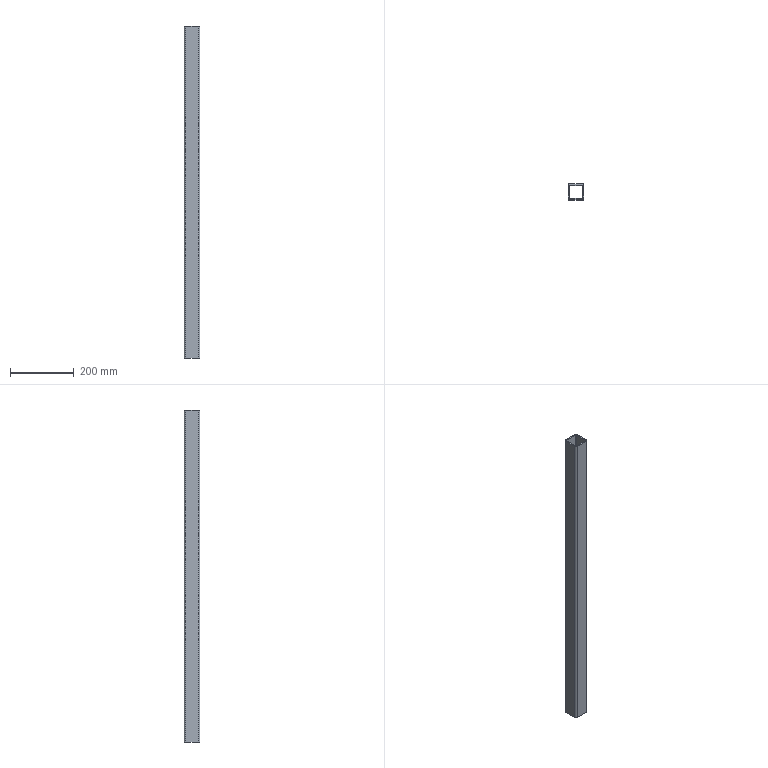Part | STEP file | Square steel 50×50×1400 | 1 solid | 18 faces | box 50 x 50 x 1040 mm | volume 744014 mm3 | plane 10 | cylinder 8 | commonest cylinder face diameters 2 x4 10 x4
STEP:
#1=CARTESIAN_POINT('',(0.,0.,0.));
#2=DIRECTION('',(0.,0.,1.));
#3=DIRECTION('',(1.,0.,0.));
#4=AXIS2_PLACEMENT_3D('',#1,#2,#3);
#5=CARTESIAN_POINT('',(-25.,-20.,520.));
#6=VERTEX_POINT('',#5);
#7=CARTESIAN_POINT('',(-20.,-25.,520.));
#8=VERTEX_POINT('',#7);
#9=CARTESIAN_POINT('',(-20.,-20.,520.));
#10=DIRECTION('',(0.,0.,1.));
#11=DIRECTION('',(1.,0.,0.));
#12=AXIS2_PLACEMENT_3D('',#9,#10,#11);
#13=CIRCLE('',#12,5.);
#14=CARTESIAN_POINT('',(-20.,-20.,520.));
#15=DIRECTION('',(0.,0.,1.));
#16=DIRECTION('',(1.,0.,0.));
#17=AXIS2_PLACEMENT_3D('',#14,#15,#16);
#18=PLANE('',#17);
#19=CARTESIAN_POINT('',(0.,0.));
#20=DIRECTION('',(1.,0.));
#21=AXIS2_PLACEMENT_2D('',#19,#20);
#22=CIRCLE('',#21,5.);
#23=(GEOMETRIC_REPRESENTATION_CONTEXT(2)PARAMETRIC_REPRESENTATION_CONTEXT()REPRESENTATION_CONTEXT('',''));
#24=DEFINITIONAL_REPRESENTATION('',(#22),#23);
#25=PCURVE('',#18,#24);
#26=CARTESIAN_POINT('',(-20.,-20.,520.));
#27=DIRECTION('',(0.,0.,-1.));
#28=DIRECTION('',(-1.,0.,0.));
#29=AXIS2_PLACEMENT_3D('',#26,#27,#28);
#30=CYLINDRICAL_SURFACE('',#29,5.);
#31=CARTESIAN_POINT('',(9.425,0.));
#32=DIRECTION('',(-1.,0.));
#33=VECTOR('',#32,1.);
#34=LINE('',#31,#33);
#35=(GEOMETRIC_REPRESENTATION_CONTEXT(2)PARAMETRIC_REPRESENTATION_CONTEXT()REPRESENTATION_CONTEXT('',''));
#36=DEFINITIONAL_REPRESENTATION('',(#34),#35);
#37=PCURVE('',#30,#36);
#38=SURFACE_CURVE('',#13,(#25,#37),.PCURVE_S1.);
#39=EDGE_CURVE('',#6,#8,#38,.T.);
#40=ORIENTED_EDGE('',*,*,#39,.T.);
#41=CARTESIAN_POINT('',(20.,-25.,520.));
#42=VERTEX_POINT('',#41);
#43=CARTESIAN_POINT('',(-20.,-25.,520.));
#44=DIRECTION('',(1.,0.,0.));
#45=VECTOR('',#44,1.);
#46=LINE('',#43,#45);
#47=CARTESIAN_POINT('',(0.,-5.));
#48=DIRECTION('',(1.,0.));
#49=VECTOR('',#48,1.);
#50=LINE('',#47,#49);
#51=(GEOMETRIC_REPRESENTATION_CONTEXT(2)PARAMETRIC_REPRESENTATION_CONTEXT()REPRESENTATION_CONTEXT('',''));
#52=DEFINITIONAL_REPRESENTATION('',(#50),#51);
#53=PCURVE('',#18,#52);
#54=CARTESIAN_POINT('',(-20.,-25.,520.));
#55=DIRECTION('',(0.,1.,0.));
#56=DIRECTION('',(0.,0.,1.));
#57=AXIS2_PLACEMENT_3D('',#54,#55,#56);
#58=PLANE('',#57);
#59=CARTESIAN_POINT('',(0.,0.));
#60=DIRECTION('',(0.,1.));
#61=VECTOR('',#60,1.);
#62=LINE('',#59,#61);
#63=(GEOMETRIC_REPRESENTATION_CONTEXT(2)PARAMETRIC_REPRESENTATION_CONTEXT()REPRESENTATION_CONTEXT('',''));
#64=DEFINITIONAL_REPRESENTATION('',(#62),#63);
#65=PCURVE('',#58,#64);
#66=SURFACE_CURVE('',#46,(#53,#65),.PCURVE_S1.);
#67=EDGE_CURVE('',#8,#42,#66,.T.);
#68=ORIENTED_EDGE('',*,*,#67,.T.);
#69=CARTESIAN_POINT('',(25.,-20.,520.));
#70=VERTEX_POINT('',#69);
#71=CARTESIAN_POINT('',(20.,-20.,520.));
#72=DIRECTION('',(0.,0.,1.));
#73=DIRECTION('',(-1.,0.,0.));
#74=AXIS2_PLACEMENT_3D('',#71,#72,#73);
#75=CIRCLE('',#74,5.);
#76=CARTESIAN_POINT('',(40.,0.));
#77=DIRECTION('',(-1.,0.));
#78=AXIS2_PLACEMENT_2D('',#76,#77);
#79=CIRCLE('',#78,5.);
#80=(GEOMETRIC_REPRESENTATION_CONTEXT(2)PARAMETRIC_REPRESENTATION_CONTEXT()REPRESENTATION_CONTEXT('',''));
#81=DEFINITIONAL_REPRESENTATION('',(#79),#80);
#82=PCURVE('',#18,#81);
#83=CARTESIAN_POINT('',(20.,-20.,520.));
#84=DIRECTION('',(0.,0.,-1.));
#85=DIRECTION('',(-1.,0.,0.));
#86=AXIS2_PLACEMENT_3D('',#83,#84,#85);
#87=CYLINDRICAL_SURFACE('',#86,5.);
#88=CARTESIAN_POINT('',(6.283,0.));
#89=DIRECTION('',(-1.,0.));
#90=VECTOR('',#89,1.);
#91=LINE('',#88,#90);
#92=(GEOMETRIC_REPRESENTATION_CONTEXT(2)PARAMETRIC_REPRESENTATION_CONTEXT()REPRESENTATION_CONTEXT('',''));
#93=DEFINITIONAL_REPRESENTATION('',(#91),#92);
#94=PCURVE('',#87,#93);
#95=SURFACE_CURVE('',#75,(#82,#94),.PCURVE_S1.);
#96=EDGE_CURVE('',#42,#70,#95,.T.);
#97=ORIENTED_EDGE('',*,*,#96,.T.);
#98=CARTESIAN_POINT('',(25.,20.,520.));
#99=VERTEX_POINT('',#98);
#100=CARTESIAN_POINT('',(25.,20.,520.));
#101=DIRECTION('',(0.,1.,0.));
#102=VECTOR('',#101,1.);
#103=LINE('',#100,#102);
#104=CARTESIAN_POINT('',(45.,40.));
#105=DIRECTION('',(0.,1.));
#106=VECTOR('',#105,1.);
#107=LINE('',#104,#106);
#108=(GEOMETRIC_REPRESENTATION_CONTEXT(2)PARAMETRIC_REPRESENTATION_CONTEXT()REPRESENTATION_CONTEXT('',''));
#109=DEFINITIONAL_REPRESENTATION('',(#107),#108);
#110=PCURVE('',#18,#109);
#111=CARTESIAN_POINT('',(25.,20.,520.));
#112=DIRECTION('',(-1.,0.,0.));
#113=DIRECTION('',(0.,-1.,0.));
#114=AXIS2_PLACEMENT_3D('',#111,#112,#113);
#115=PLANE('',#114);
#116=CARTESIAN_POINT('',(0.,0.));
#117=DIRECTION('',(-1.,0.));
#118=VECTOR('',#117,1.);
#119=LINE('',#116,#118);
#120=(GEOMETRIC_REPRESENTATION_CONTEXT(2)PARAMETRIC_REPRESENTATION_CONTEXT()REPRESENTATION_CONTEXT('',''));
#121=DEFINITIONAL_REPRESENTATION('',(#119),#120);
#122=PCURVE('',#115,#121);
#123=SURFACE_CURVE('',#103,(#110,#122),.PCURVE_S1.);
#124=EDGE_CURVE('',#70,#99,#123,.T.);
#125=ORIENTED_EDGE('',*,*,#124,.T.);
#126=CARTESIAN_POINT('',(20.,25.,520.));
#127=VERTEX_POINT('',#126);
#128=CARTESIAN_POINT('',(20.,20.,520.));
#129=DIRECTION('',(0.,0.,1.));
#130=DIRECTION('',(1.,0.,0.));
#131=AXIS2_PLACEMENT_3D('',#128,#129,#130);
#132=CIRCLE('',#131,5.);
#133=CARTESIAN_POINT('',(40.,40.));
#134=DIRECTION('',(1.,0.));
#135=AXIS2_PLACEMENT_2D('',#133,#134);
#136=CIRCLE('',#135,5.);
#137=(GEOMETRIC_REPRESENTATION_CONTEXT(2)PARAMETRIC_REPRESENTATION_CONTEXT()REPRESENTATION_CONTEXT('',''));
#138=DEFINITIONAL_REPRESENTATION('',(#136),#137);
#139=PCURVE('',#18,#138);
#140=CARTESIAN_POINT('',(20.,20.,520.));
#141=DIRECTION('',(0.,0.,-1.));
#142=DIRECTION('',(-1.,0.,0.));
#143=AXIS2_PLACEMENT_3D('',#140,#141,#142);
#144=CYLINDRICAL_SURFACE('',#143,5.);
#145=CARTESIAN_POINT('',(3.142,0.));
#146=DIRECTION('',(-1.,0.));
#147=VECTOR('',#146,1.);
#148=LINE('',#145,#147);
#149=(GEOMETRIC_REPRESENTATION_CONTEXT(2)PARAMETRIC_REPRESENTATION_CONTEXT()REPRESENTATION_CONTEXT('',''));
#150=DEFINITIONAL_REPRESENTATION('',(#148),#149);
#151=PCURVE('',#144,#150);
#152=SURFACE_CURVE('',#132,(#139,#151),.PCURVE_S1.);
#153=EDGE_CURVE('',#99,#127,#152,.T.);
#154=ORIENTED_EDGE('',*,*,#153,.T.);
#155=CARTESIAN_POINT('',(-20.,25.,520.));
#156=VERTEX_POINT('',#155);
#157=CARTESIAN_POINT('',(-20.,25.,520.));
#158=DIRECTION('',(-1.,0.,0.));
#159=VECTOR('',#158,1.);
#160=LINE('',#157,#159);
#161=CARTESIAN_POINT('',(0.,45.));
#162=DIRECTION('',(-1.,0.));
#163=VECTOR('',#162,1.);
#164=LINE('',#161,#163);
#165=(GEOMETRIC_REPRESENTATION_CONTEXT(2)PARAMETRIC_REPRESENTATION_CONTEXT()REPRESENTATION_CONTEXT('',''));
#166=DEFINITIONAL_REPRESENTATION('',(#164),#165);
#167=PCURVE('',#18,#166);
#168=CARTESIAN_POINT('',(-20.,25.,520.));
#169=DIRECTION('',(0.,-1.,0.));
#170=DIRECTION('',(0.,0.,-1.));
#171=AXIS2_PLACEMENT_3D('',#168,#169,#170);
#172=PLANE('',#171);
#173=CARTESIAN_POINT('',(0.,0.));
#174=DIRECTION('',(0.,-1.));
#175=VECTOR('',#174,1.);
#176=LINE('',#173,#175);
#177=(GEOMETRIC_REPRESENTATION_CONTEXT(2)PARAMETRIC_REPRESENTATION_CONTEXT()REPRESENTATION_CONTEXT('',''));
#178=DEFINITIONAL_REPRESENTATION('',(#176),#177);
#179=PCURVE('',#172,#178);
#180=SURFACE_CURVE('',#160,(#167,#179),.PCURVE_S1.);
#181=EDGE_CURVE('',#127,#156,#180,.T.);
#182=ORIENTED_EDGE('',*,*,#181,.T.);
#183=CARTESIAN_POINT('',(-25.,20.,520.));
#184=VERTEX_POINT('',#183);
#185=CARTESIAN_POINT('',(-20.,20.,520.));
#186=DIRECTION('',(0.,0.,1.));
#187=DIRECTION('',(-1.,0.,0.));
#188=AXIS2_PLACEMENT_3D('',#185,#186,#187);
#189=CIRCLE('',#188,5.);
#190=CARTESIAN_POINT('',(0.,40.));
#191=DIRECTION('',(-1.,0.));
#192=AXIS2_PLACEMENT_2D('',#190,#191);
#193=CIRCLE('',#192,5.);
#194=(GEOMETRIC_REPRESENTATION_CONTEXT(2)PARAMETRIC_REPRESENTATION_CONTEXT()REPRESENTATION_CONTEXT('',''));
#195=DEFINITIONAL_REPRESENTATION('',(#193),#194);
#196=PCURVE('',#18,#195);
#197=CARTESIAN_POINT('',(-20.,20.,520.));
#198=DIRECTION('',(0.,0.,-1.));
#199=DIRECTION('',(-1.,0.,0.));
#200=AXIS2_PLACEMENT_3D('',#197,#198,#199);
#201=CYLINDRICAL_SURFACE('',#200,5.);
#202=CARTESIAN_POINT('',(6.283,0.));
#203=DIRECTION('',(-1.,0.));
#204=VECTOR('',#203,1.);
#205=LINE('',#202,#204);
#206=(GEOMETRIC_REPRESENTATION_CONTEXT(2)PARAMETRIC_REPRESENTATION_CONTEXT()REPRESENTATION_CONTEXT('',''));
#207=DEFINITIONAL_REPRESENTATION('',(#205),#206);
#208=PCURVE('',#201,#207);
#209=SURFACE_CURVE('',#189,(#196,#208),.PCURVE_S1.);
#210=EDGE_CURVE('',#156,#184,#209,.T.);
#211=ORIENTED_EDGE('',*,*,#210,.T.);
#212=CARTESIAN_POINT('',(-25.,20.,520.));
#213=DIRECTION('',(0.,-1.,0.));
#214=VECTOR('',#213,1.);
#215=LINE('',#212,#214);
#216=CARTESIAN_POINT('',(-5.,40.));
#217=DIRECTION('',(0.,-1.));
#218=VECTOR('',#217,1.);
#219=LINE('',#216,#218);
#220=(GEOMETRIC_REPRESENTATION_CONTEXT(2)PARAMETRIC_REPRESENTATION_CONTEXT()REPRESENTATION_CONTEXT('',''));
#221=DEFINITIONAL_REPRESENTATION('',(#219),#220);
#222=PCURVE('',#18,#221);
#223=CARTESIAN_POINT('',(-25.,20.,520.));
#224=DIRECTION('',(1.,0.,0.));
#225=DIRECTION('',(0.,1.,0.));
#226=AXIS2_PLACEMENT_3D('',#223,#224,#225);
#227=PLANE('',#226);
#228=CARTESIAN_POINT('',(0.,0.));
#229=DIRECTION('',(-1.,0.));
#230=VECTOR('',#229,1.);
#231=LINE('',#228,#230);
#232=(GEOMETRIC_REPRESENTATION_CONTEXT(2)PARAMETRIC_REPRESENTATION_CONTEXT()REPRESENTATION_CONTEXT('',''));
#233=DEFINITIONAL_REPRESENTATION('',(#231),#232);
#234=PCURVE('',#227,#233);
#235=SURFACE_CURVE('',#215,(#222,#234),.PCURVE_S1.);
#236=EDGE_CURVE('',#184,#6,#235,.T.);
#237=ORIENTED_EDGE('',*,*,#236,.T.);
#238=EDGE_LOOP('',(#40,#68,#97,#125,#154,#182,#211,#237));
#239=FACE_BOUND('',#238,.T.);
#240=CARTESIAN_POINT('',(-21.,20.,520.));
#241=VERTEX_POINT('',#240);
#242=CARTESIAN_POINT('',(-21.,-20.,520.));
#243=VERTEX_POINT('',#242);
#244=CARTESIAN_POINT('',(-21.,20.,520.));
#245=DIRECTION('',(0.,-1.,0.));
#246=VECTOR('',#245,1.);
#247=LINE('',#244,#246);
#248=CARTESIAN_POINT('',(-1.,40.));
#249=DIRECTION('',(0.,-1.));
#250=VECTOR('',#249,1.);
#251=LINE('',#248,#250);
#252=(GEOMETRIC_REPRESENTATION_CONTEXT(2)PARAMETRIC_REPRESENTATION_CONTEXT()REPRESENTATION_CONTEXT('',''));
#253=DEFINITIONAL_REPRESENTATION('',(#251),#252);
#254=PCURVE('',#18,#253);
#255=CARTESIAN_POINT('',(-21.,20.,520.));
#256=DIRECTION('',(1.,0.,0.));
#257=DIRECTION('',(0.,1.,0.));
#258=AXIS2_PLACEMENT_3D('',#255,#256,#257);
#259=PLANE('',#258);
#260=CARTESIAN_POINT('',(0.,0.));
#261=DIRECTION('',(-1.,0.));
#262=VECTOR('',#261,1.);
#263=LINE('',#260,#262);
#264=(GEOMETRIC_REPRESENTATION_CONTEXT(2)PARAMETRIC_REPRESENTATION_CONTEXT()REPRESENTATION_CONTEXT('',''));
#265=DEFINITIONAL_REPRESENTATION('',(#263),#264);
#266=PCURVE('',#259,#265);
#267=SURFACE_CURVE('',#247,(#254,#266),.PCURVE_S1.);
#268=EDGE_CURVE('',#241,#243,#267,.T.);
#269=ORIENTED_EDGE('',*,*,#268,.F.);
#270=CARTESIAN_POINT('',(-20.,21.,520.));
#271=VERTEX_POINT('',#270);
#272=CARTESIAN_POINT('',(-20.,20.,520.));
#273=DIRECTION('',(0.,0.,1.));
#274=DIRECTION('',(-1.,0.,0.));
#275=AXIS2_PLACEMENT_3D('',#272,#273,#274);
#276=CIRCLE('',#275,1.);
#277=CARTESIAN_POINT('',(0.,40.));
#278=DIRECTION('',(-1.,0.));
#279=AXIS2_PLACEMENT_2D('',#277,#278);
#280=CIRCLE('',#279,1.);
#281=(GEOMETRIC_REPRESENTATION_CONTEXT(2)PARAMETRIC_REPRESENTATION_CONTEXT()REPRESENTATION_CONTEXT('',''));
#282=DEFINITIONAL_REPRESENTATION('',(#280),#281);
#283=PCURVE('',#18,#282);
#284=CARTESIAN_POINT('',(-20.,20.,520.));
#285=DIRECTION('',(0.,0.,-1.));
#286=DIRECTION('',(-1.,0.,0.));
#287=AXIS2_PLACEMENT_3D('',#284,#285,#286);
#288=CYLINDRICAL_SURFACE('',#287,1.);
#289=CARTESIAN_POINT('',(6.283,0.));
#290=DIRECTION('',(-1.,0.));
#291=VECTOR('',#290,1.);
#292=LINE('',#289,#291);
#293=(GEOMETRIC_REPRESENTATION_CONTEXT(2)PARAMETRIC_REPRESENTATION_CONTEXT()REPRESENTATION_CONTEXT('',''));
#294=DEFINITIONAL_REPRESENTATION('',(#292),#293);
#295=PCURVE('',#288,#294);
#296=SURFACE_CURVE('',#276,(#283,#295),.PCURVE_S1.);
#297=EDGE_CURVE('',#271,#241,#296,.T.);
#298=ORIENTED_EDGE('',*,*,#297,.F.);
#299=CARTESIAN_POINT('',(20.,21.,520.));
#300=VERTEX_POINT('',#299);
#301=CARTESIAN_POINT('',(-20.,21.,520.));
#302=DIRECTION('',(-1.,0.,0.));
#303=VECTOR('',#302,1.);
#304=LINE('',#301,#303);
#305=CARTESIAN_POINT('',(0.,41.));
#306=DIRECTION('',(-1.,0.));
#307=VECTOR('',#306,1.);
#308=LINE('',#305,#307);
#309=(GEOMETRIC_REPRESENTATION_CONTEXT(2)PARAMETRIC_REPRESENTATION_CONTEXT()REPRESENTATION_CONTEXT('',''));
#310=DEFINITIONAL_REPRESENTATION('',(#308),#309);
#311=PCURVE('',#18,#310);
#312=CARTESIAN_POINT('',(-20.,21.,520.));
#313=DIRECTION('',(0.,-1.,0.));
#314=DIRECTION('',(0.,0.,-1.));
#315=AXIS2_PLACEMENT_3D('',#312,#313,#314);
#316=PLANE('',#315);
#317=CARTESIAN_POINT('',(0.,0.));
#318=DIRECTION('',(0.,-1.));
#319=VECTOR('',#318,1.);
#320=LINE('',#317,#319);
#321=(GEOMETRIC_REPRESENTATION_CONTEXT(2)PARAMETRIC_REPRESENTATION_CONTEXT()REPRESENTATION_CONTEXT('',''));
#322=DEFINITIONAL_REPRESENTATION('',(#320),#321);
#323=PCURVE('',#316,#322);
#324=SURFACE_CURVE('',#304,(#311,#323),.PCURVE_S1.);
#325=EDGE_CURVE('',#300,#271,#324,.T.);
#326=ORIENTED_EDGE('',*,*,#325,.F.);
#327=CARTESIAN_POINT('',(21.,20.,520.));
#328=VERTEX_POINT('',#327);
#329=CARTESIAN_POINT('',(20.,20.,520.));
#330=DIRECTION('',(0.,0.,1.));
#331=DIRECTION('',(1.,0.,0.));
#332=AXIS2_PLACEMENT_3D('',#329,#330,#331);
#333=CIRCLE('',#332,1.);
#334=CARTESIAN_POINT('',(40.,40.));
#335=DIRECTION('',(1.,0.));
#336=AXIS2_PLACEMENT_2D('',#334,#335);
#337=CIRCLE('',#336,1.);
#338=(GEOMETRIC_REPRESENTATION_CONTEXT(2)PARAMETRIC_REPRESENTATION_CONTEXT()REPRESENTATION_CONTEXT('',''));
#339=DEFINITIONAL_REPRESENTATION('',(#337),#338);
#340=PCURVE('',#18,#339);
#341=CARTESIAN_POINT('',(20.,20.,520.));
#342=DIRECTION('',(0.,0.,-1.));
#343=DIRECTION('',(-1.,0.,0.));
#344=AXIS2_PLACEMENT_3D('',#341,#342,#343);
#345=CYLINDRICAL_SURFACE('',#344,1.);
#346=CARTESIAN_POINT('',(3.142,0.));
#347=DIRECTION('',(-1.,0.));
#348=VECTOR('',#347,1.);
#349=LINE('',#346,#348);
#350=(GEOMETRIC_REPRESENTATION_CONTEXT(2)PARAMETRIC_REPRESENTATION_CONTEXT()REPRESENTATION_CONTEXT('',''));
#351=DEFINITIONAL_REPRESENTATION('',(#349),#350);
#352=PCURVE('',#345,#351);
#353=SURFACE_CURVE('',#333,(#340,#352),.PCURVE_S1.);
#354=EDGE_CURVE('',#328,#300,#353,.T.);
#355=ORIENTED_EDGE('',*,*,#354,.F.);
#356=CARTESIAN_POINT('',(21.,-20.,520.));
#357=VERTEX_POINT('',#356);
#358=CARTESIAN_POINT('',(21.,20.,520.));
#359=DIRECTION('',(0.,1.,0.));
#360=VECTOR('',#359,1.);
#361=LINE('',#358,#360);
#362=CARTESIAN_POINT('',(41.,40.));
#363=DIRECTION('',(0.,1.));
#364=VECTOR('',#363,1.);
#365=LINE('',#362,#364);
#366=(GEOMETRIC_REPRESENTATION_CONTEXT(2)PARAMETRIC_REPRESENTATION_CONTEXT()REPRESENTATION_CONTEXT('',''));
#367=DEFINITIONAL_REPRESENTATION('',(#365),#366);
#368=PCURVE('',#18,#367);
#369=CARTESIAN_POINT('',(21.,20.,520.));
#370=DIRECTION('',(-1.,0.,0.));
#371=DIRECTION('',(0.,0.,1.));
#372=AXIS2_PLACEMENT_3D('',#369,#370,#371);
#373=PLANE('',#372);
#374=CARTESIAN_POINT('',(0.,0.));
#375=DIRECTION('',(0.,1.));
#376=VECTOR('',#375,1.);
#377=LINE('',#374,#376);
#378=(GEOMETRIC_REPRESENTATION_CONTEXT(2)PARAMETRIC_REPRESENTATION_CONTEXT()REPRESENTATION_CONTEXT('',''));
#379=DEFINITIONAL_REPRESENTATION('',(#377),#378);
#380=PCURVE('',#373,#379);
#381=SURFACE_CURVE('',#361,(#368,#380),.PCURVE_S1.);
#382=EDGE_CURVE('',#357,#328,#381,.T.);
#383=ORIENTED_EDGE('',*,*,#382,.F.);
#384=CARTESIAN_POINT('',(20.,-21.,520.));
#385=VERTEX_POINT('',#384);
#386=CARTESIAN_POINT('',(20.,-20.,520.));
#387=DIRECTION('',(0.,0.,1.));
#388=DIRECTION('',(-1.,0.,0.));
#389=AXIS2_PLACEMENT_3D('',#386,#387,#388);
#390=CIRCLE('',#389,1.);
#391=CARTESIAN_POINT('',(40.,0.));
#392=DIRECTION('',(-1.,0.));
#393=AXIS2_PLACEMENT_2D('',#391,#392);
#394=CIRCLE('',#393,1.);
#395=(GEOMETRIC_REPRESENTATION_CONTEXT(2)PARAMETRIC_REPRESENTATION_CONTEXT()REPRESENTATION_CONTEXT('',''));
#396=DEFINITIONAL_REPRESENTATION('',(#394),#395);
#397=PCURVE('',#18,#396);
#398=CARTESIAN_POINT('',(20.,-20.,520.));
#399=DIRECTION('',(0.,0.,-1.));
#400=DIRECTION('',(-1.,0.,0.));
#401=AXIS2_PLACEMENT_3D('',#398,#399,#400);
#402=CYLINDRICAL_SURFACE('',#401,1.);
#403=CARTESIAN_POINT('',(6.283,0.));
#404=DIRECTION('',(-1.,0.));
#405=VECTOR('',#404,1.);
#406=LINE('',#403,#405);
#407=(GEOMETRIC_REPRESENTATION_CONTEXT(2)PARAMETRIC_REPRESENTATION_CONTEXT()REPRESENTATION_CONTEXT('',''));
#408=DEFINITIONAL_REPRESENTATION('',(#406),#407);
#409=PCURVE('',#402,#408);
#410=SURFACE_CURVE('',#390,(#397,#409),.PCURVE_S1.);
#411=EDGE_CURVE('',#385,#357,#410,.T.);
#412=ORIENTED_EDGE('',*,*,#411,.F.);
#413=CARTESIAN_POINT('',(-20.,-21.,520.));
#414=VERTEX_POINT('',#413);
#415=CARTESIAN_POINT('',(-20.,-21.,520.));
#416=DIRECTION('',(1.,0.,0.));
#417=VECTOR('',#416,1.);
#418=LINE('',#415,#417);
#419=CARTESIAN_POINT('',(0.,-1.));
#420=DIRECTION('',(1.,0.));
#421=VECTOR('',#420,1.);
#422=LINE('',#419,#421);
#423=(GEOMETRIC_REPRESENTATION_CONTEXT(2)PARAMETRIC_REPRESENTATION_CONTEXT()REPRESENTATION_CONTEXT('',''));
#424=DEFINITIONAL_REPRESENTATION('',(#422),#423);
#425=PCURVE('',#18,#424);
#426=CARTESIAN_POINT('',(-20.,-21.,520.));
#427=DIRECTION('',(0.,1.,0.));
#428=DIRECTION('',(0.,0.,1.));
#429=AXIS2_PLACEMENT_3D('',#426,#427,#428);
#430=PLANE('',#429);
#431=CARTESIAN_POINT('',(0.,0.));
#432=DIRECTION('',(0.,1.));
#433=VECTOR('',#432,1.);
#434=LINE('',#431,#433);
#435=(GEOMETRIC_REPRESENTATION_CONTEXT(2)PARAMETRIC_REPRESENTATION_CONTEXT()REPRESENTATION_CONTEXT('',''));
#436=DEFINITIONAL_REPRESENTATION('',(#434),#435);
#437=PCURVE('',#430,#436);
#438=SURFACE_CURVE('',#418,(#425,#437),.PCURVE_S1.);
#439=EDGE_CURVE('',#414,#385,#438,.T.);
#440=ORIENTED_EDGE('',*,*,#439,.F.);
#441=CARTESIAN_POINT('',(-20.,-20.,520.));
#442=DIRECTION('',(0.,0.,1.));
#443=DIRECTION('',(1.,0.,0.));
#444=AXIS2_PLACEMENT_3D('',#441,#442,#443);
#445=CIRCLE('',#444,1.);
#446=CARTESIAN_POINT('',(0.,0.));
#447=DIRECTION('',(1.,0.));
#448=AXIS2_PLACEMENT_2D('',#446,#447);
#449=CIRCLE('',#448,1.);
#450=(GEOMETRIC_REPRESENTATION_CONTEXT(2)PARAMETRIC_REPRESENTATION_CONTEXT()REPRESENTATION_CONTEXT('',''));
#451=DEFINITIONAL_REPRESENTATION('',(#449),#450);
#452=PCURVE('',#18,#451);
#453=CARTESIAN_POINT('',(-20.,-20.,520.));
#454=DIRECTION('',(0.,0.,-1.));
#455=DIRECTION('',(-1.,0.,0.));
#456=AXIS2_PLACEMENT_3D('',#453,#454,#455);
#457=CYLINDRICAL_SURFACE('',#456,1.);
#458=CARTESIAN_POINT('',(9.425,0.));
#459=DIRECTION('',(-1.,0.));
#460=VECTOR('',#459,1.);
#461=LINE('',#458,#460);
#462=(GEOMETRIC_REPRESENTATION_CONTEXT(2)PARAMETRIC_REPRESENTATION_CONTEXT()REPRESENTATION_CONTEXT('',''));
#463=DEFINITIONAL_REPRESENTATION('',(#461),#462);
#464=PCURVE('',#457,#463);
#465=SURFACE_CURVE('',#445,(#452,#464),.PCURVE_S1.);
#466=EDGE_CURVE('',#243,#414,#465,.T.);
#467=ORIENTED_EDGE('',*,*,#466,.F.);
#468=EDGE_LOOP('',(#269,#298,#326,#355,#383,#412,#440,#467));
#469=FACE_BOUND('',#468,.T.);
#470=ADVANCED_FACE('',(#239,#469),#18,.T.);
#471=CARTESIAN_POINT('',(-25.,-20.,-520.));
#472=VERTEX_POINT('',#471);
#473=CARTESIAN_POINT('',(-20.,-25.,-520.));
#474=VERTEX_POINT('',#473);
#475=CARTESIAN_POINT('',(-20.,-20.,-520.));
#476=DIRECTION('',(0.,0.,1.));
#477=DIRECTION('',(1.,0.,0.));
#478=AXIS2_PLACEMENT_3D('',#475,#476,#477);
#479=CIRCLE('',#478,5.);
#480=CARTESIAN_POINT('',(-20.,-20.,-520.));
#481=DIRECTION('',(0.,0.,1.));
#482=DIRECTION('',(1.,0.,0.));
#483=AXIS2_PLACEMENT_3D('',#480,#481,#482);
#484=PLANE('',#483);
#485=CARTESIAN_POINT('',(0.,0.));
#486=DIRECTION('',(1.,0.));
#487=AXIS2_PLACEMENT_2D('',#485,#486);
#488=CIRCLE('',#487,5.);
#489=(GEOMETRIC_REPRESENTATION_CONTEXT(2)PARAMETRIC_REPRESENTATION_CONTEXT()REPRESENTATION_CONTEXT('',''));
#490=DEFINITIONAL_REPRESENTATION('',(#488),#489);
#491=PCURVE('',#484,#490);
#492=CARTESIAN_POINT('',(9.425,1040.));
#493=DIRECTION('',(-1.,0.));
#494=VECTOR('',#493,1.);
#495=LINE('',#492,#494);
#496=(GEOMETRIC_REPRESENTATION_CONTEXT(2)PARAMETRIC_REPRESENTATION_CONTEXT()REPRESENTATION_CONTEXT('',''));
#497=DEFINITIONAL_REPRESENTATION('',(#495),#496);
#498=PCURVE('',#30,#497);
#499=SURFACE_CURVE('',#479,(#491,#498),.PCURVE_S1.);
#500=EDGE_CURVE('',#472,#474,#499,.T.);
#501=ORIENTED_EDGE('',*,*,#500,.F.);
#502=CARTESIAN_POINT('',(-25.,20.,-520.));
#503=VERTEX_POINT('',#502);
#504=CARTESIAN_POINT('',(-25.,20.,-520.));
#505=DIRECTION('',(0.,-1.,0.));
#506=VECTOR('',#505,1.);
#507=LINE('',#504,#506);
#508=CARTESIAN_POINT('',(-5.,40.));
#509=DIRECTION('',(0.,-1.));
#510=VECTOR('',#509,1.);
#511=LINE('',#508,#510);
#512=(GEOMETRIC_REPRESENTATION_CONTEXT(2)PARAMETRIC_REPRESENTATION_CONTEXT()REPRESENTATION_CONTEXT('',''));
#513=DEFINITIONAL_REPRESENTATION('',(#511),#512);
#514=PCURVE('',#484,#513);
#515=CARTESIAN_POINT('',(0.,-1040.));
#516=DIRECTION('',(-1.,0.));
#517=VECTOR('',#516,1.);
#518=LINE('',#515,#517);
#519=(GEOMETRIC_REPRESENTATION_CONTEXT(2)PARAMETRIC_REPRESENTATION_CONTEXT()REPRESENTATION_CONTEXT('',''));
#520=DEFINITIONAL_REPRESENTATION('',(#518),#519);
#521=PCURVE('',#227,#520);
#522=SURFACE_CURVE('',#507,(#514,#521),.PCURVE_S1.);
#523=EDGE_CURVE('',#503,#472,#522,.T.);
#524=ORIENTED_EDGE('',*,*,#523,.F.);
#525=CARTESIAN_POINT('',(-20.,25.,-520.));
#526=VERTEX_POINT('',#525);
#527=CARTESIAN_POINT('',(-20.,20.,-520.));
#528=DIRECTION('',(0.,0.,1.));
#529=DIRECTION('',(-1.,0.,0.));
#530=AXIS2_PLACEMENT_3D('',#527,#528,#529);
#531=CIRCLE('',#530,5.);
#532=CARTESIAN_POINT('',(0.,40.));
#533=DIRECTION('',(-1.,0.));
#534=AXIS2_PLACEMENT_2D('',#532,#533);
#535=CIRCLE('',#534,5.);
#536=(GEOMETRIC_REPRESENTATION_CONTEXT(2)PARAMETRIC_REPRESENTATION_CONTEXT()REPRESENTATION_CONTEXT('',''));
#537=DEFINITIONAL_REPRESENTATION('',(#535),#536);
#538=PCURVE('',#484,#537);
#539=CARTESIAN_POINT('',(6.283,1040.));
#540=DIRECTION('',(-1.,0.));
#541=VECTOR('',#540,1.);
#542=LINE('',#539,#541);
#543=(GEOMETRIC_REPRESENTATION_CONTEXT(2)PARAMETRIC_REPRESENTATION_CONTEXT()REPRESENTATION_CONTEXT('',''));
#544=DEFINITIONAL_REPRESENTATION('',(#542),#543);
#545=PCURVE('',#201,#544);
#546=SURFACE_CURVE('',#531,(#538,#545),.PCURVE_S1.);
#547=EDGE_CURVE('',#526,#503,#546,.T.);
#548=ORIENTED_EDGE('',*,*,#547,.F.);
#549=CARTESIAN_POINT('',(20.,25.,-520.));
#550=VERTEX_POINT('',#549);
#551=CARTESIAN_POINT('',(-20.,25.,-520.));
#552=DIRECTION('',(-1.,0.,0.));
#553=VECTOR('',#552,1.);
#554=LINE('',#551,#553);
#555=CARTESIAN_POINT('',(0.,45.));
#556=DIRECTION('',(-1.,0.));
#557=VECTOR('',#556,1.);
#558=LINE('',#555,#557);
#559=(GEOMETRIC_REPRESENTATION_CONTEXT(2)PARAMETRIC_REPRESENTATION_CONTEXT()REPRESENTATION_CONTEXT('',''));
#560=DEFINITIONAL_REPRESENTATION('',(#558),#559);
#561=PCURVE('',#484,#560);
#562=CARTESIAN_POINT('',(1040.,0.));
#563=DIRECTION('',(0.,-1.));
#564=VECTOR('',#563,1.);
#565=LINE('',#562,#564);
#566=(GEOMETRIC_REPRESENTATION_CONTEXT(2)PARAMETRIC_REPRESENTATION_CONTEXT()REPRESENTATION_CONTEXT('',''));
#567=DEFINITIONAL_REPRESENTATION('',(#565),#566);
#568=PCURVE('',#172,#567);
#569=SURFACE_CURVE('',#554,(#561,#568),.PCURVE_S1.);
#570=EDGE_CURVE('',#550,#526,#569,.T.);
#571=ORIENTED_EDGE('',*,*,#570,.F.);
#572=CARTESIAN_POINT('',(25.,20.,-520.));
#573=VERTEX_POINT('',#572);
#574=CARTESIAN_POINT('',(20.,20.,-520.));
#575=DIRECTION('',(0.,0.,1.));
#576=DIRECTION('',(1.,0.,0.));
#577=AXIS2_PLACEMENT_3D('',#574,#575,#576);
#578=CIRCLE('',#577,5.);
#579=CARTESIAN_POINT('',(40.,40.));
#580=DIRECTION('',(1.,0.));
#581=AXIS2_PLACEMENT_2D('',#579,#580);
#582=CIRCLE('',#581,5.);
#583=(GEOMETRIC_REPRESENTATION_CONTEXT(2)PARAMETRIC_REPRESENTATION_CONTEXT()REPRESENTATION_CONTEXT('',''));
#584=DEFINITIONAL_REPRESENTATION('',(#582),#583);
#585=PCURVE('',#484,#584);
#586=CARTESIAN_POINT('',(3.142,1040.));
#587=DIRECTION('',(-1.,0.));
#588=VECTOR('',#587,1.);
#589=LINE('',#586,#588);
#590=(GEOMETRIC_REPRESENTATION_CONTEXT(2)PARAMETRIC_REPRESENTATION_CONTEXT()REPRESENTATION_CONTEXT('',''));
#591=DEFINITIONAL_REPRESENTATION('',(#589),#590);
#592=PCURVE('',#144,#591);
#593=SURFACE_CURVE('',#578,(#585,#592),.PCURVE_S1.);
#594=EDGE_CURVE('',#573,#550,#593,.T.);
#595=ORIENTED_EDGE('',*,*,#594,.F.);
#596=CARTESIAN_POINT('',(25.,-20.,-520.));
#597=VERTEX_POINT('',#596);
#598=CARTESIAN_POINT('',(25.,20.,-520.));
#599=DIRECTION('',(0.,1.,0.));
#600=VECTOR('',#599,1.);
#601=LINE('',#598,#600);
#602=CARTESIAN_POINT('',(45.,40.));
#603=DIRECTION('',(0.,1.));
#604=VECTOR('',#603,1.);
#605=LINE('',#602,#604);
#606=(GEOMETRIC_REPRESENTATION_CONTEXT(2)PARAMETRIC_REPRESENTATION_CONTEXT()REPRESENTATION_CONTEXT('',''));
#607=DEFINITIONAL_REPRESENTATION('',(#605),#606);
#608=PCURVE('',#484,#607);
#609=CARTESIAN_POINT('',(0.,-1040.));
#610=DIRECTION('',(-1.,0.));
#611=VECTOR('',#610,1.);
#612=LINE('',#609,#611);
#613=(GEOMETRIC_REPRESENTATION_CONTEXT(2)PARAMETRIC_REPRESENTATION_CONTEXT()REPRESENTATION_CONTEXT('',''));
#614=DEFINITIONAL_REPRESENTATION('',(#612),#613);
#615=PCURVE('',#115,#614);
#616=SURFACE_CURVE('',#601,(#608,#615),.PCURVE_S1.);
#617=EDGE_CURVE('',#597,#573,#616,.T.);
#618=ORIENTED_EDGE('',*,*,#617,.F.);
#619=CARTESIAN_POINT('',(20.,-25.,-520.));
#620=VERTEX_POINT('',#619);
#621=CARTESIAN_POINT('',(20.,-20.,-520.));
#622=DIRECTION('',(0.,0.,1.));
#623=DIRECTION('',(-1.,0.,0.));
#624=AXIS2_PLACEMENT_3D('',#621,#622,#623);
#625=CIRCLE('',#624,5.);
#626=CARTESIAN_POINT('',(40.,0.));
#627=DIRECTION('',(-1.,0.));
#628=AXIS2_PLACEMENT_2D('',#626,#627);
#629=CIRCLE('',#628,5.);
#630=(GEOMETRIC_REPRESENTATION_CONTEXT(2)PARAMETRIC_REPRESENTATION_CONTEXT()REPRESENTATION_CONTEXT('',''));
#631=DEFINITIONAL_REPRESENTATION('',(#629),#630);
#632=PCURVE('',#484,#631);
#633=CARTESIAN_POINT('',(6.283,1040.));
#634=DIRECTION('',(-1.,0.));
#635=VECTOR('',#634,1.);
#636=LINE('',#633,#635);
#637=(GEOMETRIC_REPRESENTATION_CONTEXT(2)PARAMETRIC_REPRESENTATION_CONTEXT()REPRESENTATION_CONTEXT('',''));
#638=DEFINITIONAL_REPRESENTATION('',(#636),#637);
#639=PCURVE('',#87,#638);
#640=SURFACE_CURVE('',#625,(#632,#639),.PCURVE_S1.);
#641=EDGE_CURVE('',#620,#597,#640,.T.);
#642=ORIENTED_EDGE('',*,*,#641,.F.);
#643=CARTESIAN_POINT('',(-20.,-25.,-520.));
#644=DIRECTION('',(1.,0.,0.));
#645=VECTOR('',#644,1.);
#646=LINE('',#643,#645);
#647=CARTESIAN_POINT('',(0.,-5.));
#648=DIRECTION('',(1.,0.));
#649=VECTOR('',#648,1.);
#650=LINE('',#647,#649);
#651=(GEOMETRIC_REPRESENTATION_CONTEXT(2)PARAMETRIC_REPRESENTATION_CONTEXT()REPRESENTATION_CONTEXT('',''));
#652=DEFINITIONAL_REPRESENTATION('',(#650),#651);
#653=PCURVE('',#484,#652);
#654=CARTESIAN_POINT('',(-1040.,0.));
#655=DIRECTION('',(0.,1.));
#656=VECTOR('',#655,1.);
#657=LINE('',#654,#656);
#658=(GEOMETRIC_REPRESENTATION_CONTEXT(2)PARAMETRIC_REPRESENTATION_CONTEXT()REPRESENTATION_CONTEXT('',''));
#659=DEFINITIONAL_REPRESENTATION('',(#657),#658);
#660=PCURVE('',#58,#659);
#661=SURFACE_CURVE('',#646,(#653,#660),.PCURVE_S1.);
#662=EDGE_CURVE('',#474,#620,#661,.T.);
#663=ORIENTED_EDGE('',*,*,#662,.F.);
#664=EDGE_LOOP('',(#501,#524,#548,#571,#595,#618,#642,#663));
#665=FACE_BOUND('',#664,.T.);
#666=CARTESIAN_POINT('',(-20.,21.,-520.));
#667=VERTEX_POINT('',#666);
#668=CARTESIAN_POINT('',(-21.,20.,-520.));
#669=VERTEX_POINT('',#668);
#670=CARTESIAN_POINT('',(-20.,20.,-520.));
#671=DIRECTION('',(0.,0.,1.));
#672=DIRECTION('',(-1.,0.,0.));
#673=AXIS2_PLACEMENT_3D('',#670,#671,#672);
#674=CIRCLE('',#673,1.);
#675=CARTESIAN_POINT('',(0.,40.));
#676=DIRECTION('',(-1.,0.));
#677=AXIS2_PLACEMENT_2D('',#675,#676);
#678=CIRCLE('',#677,1.);
#679=(GEOMETRIC_REPRESENTATION_CONTEXT(2)PARAMETRIC_REPRESENTATION_CONTEXT()REPRESENTATION_CONTEXT('',''));
#680=DEFINITIONAL_REPRESENTATION('',(#678),#679);
#681=PCURVE('',#484,#680);
#682=CARTESIAN_POINT('',(6.283,1040.));
#683=DIRECTION('',(-1.,0.));
#684=VECTOR('',#683,1.);
#685=LINE('',#682,#684);
#686=(GEOMETRIC_REPRESENTATION_CONTEXT(2)PARAMETRIC_REPRESENTATION_CONTEXT()REPRESENTATION_CONTEXT('',''));
#687=DEFINITIONAL_REPRESENTATION('',(#685),#686);
#688=PCURVE('',#288,#687);
#689=SURFACE_CURVE('',#674,(#681,#688),.PCURVE_S1.);
#690=EDGE_CURVE('',#667,#669,#689,.T.);
#691=ORIENTED_EDGE('',*,*,#690,.T.);
#692=CARTESIAN_POINT('',(-21.,-20.,-520.));
#693=VERTEX_POINT('',#692);
#694=CARTESIAN_POINT('',(-21.,20.,-520.));
#695=DIRECTION('',(0.,-1.,0.));
#696=VECTOR('',#695,1.);
#697=LINE('',#694,#696);
#698=CARTESIAN_POINT('',(-1.,40.));
#699=DIRECTION('',(0.,-1.));
#700=VECTOR('',#699,1.);
#701=LINE('',#698,#700);
#702=(GEOMETRIC_REPRESENTATION_CONTEXT(2)PARAMETRIC_REPRESENTATION_CONTEXT()REPRESENTATION_CONTEXT('',''));
#703=DEFINITIONAL_REPRESENTATION('',(#701),#702);
#704=PCURVE('',#484,#703);
#705=CARTESIAN_POINT('',(0.,-1040.));
#706=DIRECTION('',(-1.,0.));
#707=VECTOR('',#706,1.);
#708=LINE('',#705,#707);
#709=(GEOMETRIC_REPRESENTATION_CONTEXT(2)PARAMETRIC_REPRESENTATION_CONTEXT()REPRESENTATION_CONTEXT('',''));
#710=DEFINITIONAL_REPRESENTATION('',(#708),#709);
#711=PCURVE('',#259,#710);
#712=SURFACE_CURVE('',#697,(#704,#711),.PCURVE_S1.);
#713=EDGE_CURVE('',#669,#693,#712,.T.);
#714=ORIENTED_EDGE('',*,*,#713,.T.);
#715=CARTESIAN_POINT('',(-20.,-21.,-520.));
#716=VERTEX_POINT('',#715);
#717=CARTESIAN_POINT('',(-20.,-20.,-520.));
#718=DIRECTION('',(0.,0.,1.));
#719=DIRECTION('',(1.,0.,0.));
#720=AXIS2_PLACEMENT_3D('',#717,#718,#719);
#721=CIRCLE('',#720,1.);
#722=CARTESIAN_POINT('',(0.,0.));
#723=DIRECTION('',(1.,0.));
#724=AXIS2_PLACEMENT_2D('',#722,#723);
#725=CIRCLE('',#724,1.);
#726=(GEOMETRIC_REPRESENTATION_CONTEXT(2)PARAMETRIC_REPRESENTATION_CONTEXT()REPRESENTATION_CONTEXT('',''));
#727=DEFINITIONAL_REPRESENTATION('',(#725),#726);
#728=PCURVE('',#484,#727);
#729=CARTESIAN_POINT('',(9.425,1040.));
#730=DIRECTION('',(-1.,0.));
#731=VECTOR('',#730,1.);
#732=LINE('',#729,#731);
#733=(GEOMETRIC_REPRESENTATION_CONTEXT(2)PARAMETRIC_REPRESENTATION_CONTEXT()REPRESENTATION_CONTEXT('',''));
#734=DEFINITIONAL_REPRESENTATION('',(#732),#733);
#735=PCURVE('',#457,#734);
#736=SURFACE_CURVE('',#721,(#728,#735),.PCURVE_S1.);
#737=EDGE_CURVE('',#693,#716,#736,.T.);
#738=ORIENTED_EDGE('',*,*,#737,.T.);
#739=CARTESIAN_POINT('',(20.,-21.,-520.));
#740=VERTEX_POINT('',#739);
#741=CARTESIAN_POINT('',(-20.,-21.,-520.));
#742=DIRECTION('',(1.,0.,0.));
#743=VECTOR('',#742,1.);
#744=LINE('',#741,#743);
#745=CARTESIAN_POINT('',(0.,-1.));
#746=DIRECTION('',(1.,0.));
#747=VECTOR('',#746,1.);
#748=LINE('',#745,#747);
#749=(GEOMETRIC_REPRESENTATION_CONTEXT(2)PARAMETRIC_REPRESENTATION_CONTEXT()REPRESENTATION_CONTEXT('',''));
#750=DEFINITIONAL_REPRESENTATION('',(#748),#749);
#751=PCURVE('',#484,#750);
#752=CARTESIAN_POINT('',(-1040.,0.));
#753=DIRECTION('',(0.,1.));
#754=VECTOR('',#753,1.);
#755=LINE('',#752,#754);
#756=(GEOMETRIC_REPRESENTATION_CONTEXT(2)PARAMETRIC_REPRESENTATION_CONTEXT()REPRESENTATION_CONTEXT('',''));
#757=DEFINITIONAL_REPRESENTATION('',(#755),#756);
#758=PCURVE('',#430,#757);
#759=SURFACE_CURVE('',#744,(#751,#758),.PCURVE_S1.);
#760=EDGE_CURVE('',#716,#740,#759,.T.);
#761=ORIENTED_EDGE('',*,*,#760,.T.);
#762=CARTESIAN_POINT('',(21.,-20.,-520.));
#763=VERTEX_POINT('',#762);
#764=CARTESIAN_POINT('',(20.,-20.,-520.));
#765=DIRECTION('',(0.,0.,1.));
#766=DIRECTION('',(-1.,0.,0.));
#767=AXIS2_PLACEMENT_3D('',#764,#765,#766);
#768=CIRCLE('',#767,1.);
#769=CARTESIAN_POINT('',(40.,0.));
#770=DIRECTION('',(-1.,0.));
#771=AXIS2_PLACEMENT_2D('',#769,#770);
#772=CIRCLE('',#771,1.);
#773=(GEOMETRIC_REPRESENTATION_CONTEXT(2)PARAMETRIC_REPRESENTATION_CONTEXT()REPRESENTATION_CONTEXT('',''));
#774=DEFINITIONAL_REPRESENTATION('',(#772),#773);
#775=PCURVE('',#484,#774);
#776=CARTESIAN_POINT('',(6.283,1040.));
#777=DIRECTION('',(-1.,0.));
#778=VECTOR('',#777,1.);
#779=LINE('',#776,#778);
#780=(GEOMETRIC_REPRESENTATION_CONTEXT(2)PARAMETRIC_REPRESENTATION_CONTEXT()REPRESENTATION_CONTEXT('',''));
#781=DEFINITIONAL_REPRESENTATION('',(#779),#780);
#782=PCURVE('',#402,#781);
#783=SURFACE_CURVE('',#768,(#775,#782),.PCURVE_S1.);
#784=EDGE_CURVE('',#740,#763,#783,.T.);
#785=ORIENTED_EDGE('',*,*,#784,.T.);
#786=CARTESIAN_POINT('',(21.,20.,-520.));
#787=VERTEX_POINT('',#786);
#788=CARTESIAN_POINT('',(21.,20.,-520.));
#789=DIRECTION('',(0.,1.,0.));
#790=VECTOR('',#789,1.);
#791=LINE('',#788,#790);
#792=CARTESIAN_POINT('',(41.,40.));
#793=DIRECTION('',(0.,1.));
#794=VECTOR('',#793,1.);
#795=LINE('',#792,#794);
#796=(GEOMETRIC_REPRESENTATION_CONTEXT(2)PARAMETRIC_REPRESENTATION_CONTEXT()REPRESENTATION_CONTEXT('',''));
#797=DEFINITIONAL_REPRESENTATION('',(#795),#796);
#798=PCURVE('',#484,#797);
#799=CARTESIAN_POINT('',(-1040.,0.));
#800=DIRECTION('',(0.,1.));
#801=VECTOR('',#800,1.);
#802=LINE('',#799,#801);
#803=(GEOMETRIC_REPRESENTATION_CONTEXT(2)PARAMETRIC_REPRESENTATION_CONTEXT()REPRESENTATION_CONTEXT('',''));
#804=DEFINITIONAL_REPRESENTATION('',(#802),#803);
#805=PCURVE('',#373,#804);
#806=SURFACE_CURVE('',#791,(#798,#805),.PCURVE_S1.);
#807=EDGE_CURVE('',#763,#787,#806,.T.);
#808=ORIENTED_EDGE('',*,*,#807,.T.);
#809=CARTESIAN_POINT('',(20.,21.,-520.));
#810=VERTEX_POINT('',#809);
#811=CARTESIAN_POINT('',(20.,20.,-520.));
#812=DIRECTION('',(0.,0.,1.));
#813=DIRECTION('',(1.,0.,0.));
#814=AXIS2_PLACEMENT_3D('',#811,#812,#813);
#815=CIRCLE('',#814,1.);
#816=CARTESIAN_POINT('',(40.,40.));
#817=DIRECTION('',(1.,0.));
#818=AXIS2_PLACEMENT_2D('',#816,#817);
#819=CIRCLE('',#818,1.);
#820=(GEOMETRIC_REPRESENTATION_CONTEXT(2)PARAMETRIC_REPRESENTATION_CONTEXT()REPRESENTATION_CONTEXT('',''));
#821=DEFINITIONAL_REPRESENTATION('',(#819),#820);
#822=PCURVE('',#484,#821);
#823=CARTESIAN_POINT('',(3.142,1040.));
#824=DIRECTION('',(-1.,0.));
#825=VECTOR('',#824,1.);
#826=LINE('',#823,#825);
#827=(GEOMETRIC_REPRESENTATION_CONTEXT(2)PARAMETRIC_REPRESENTATION_CONTEXT()REPRESENTATION_CONTEXT('',''));
#828=DEFINITIONAL_REPRESENTATION('',(#826),#827);
#829=PCURVE('',#345,#828);
#830=SURFACE_CURVE('',#815,(#822,#829),.PCURVE_S1.);
#831=EDGE_CURVE('',#787,#810,#830,.T.);
#832=ORIENTED_EDGE('',*,*,#831,.T.);
#833=CARTESIAN_POINT('',(-20.,21.,-520.));
#834=DIRECTION('',(-1.,0.,0.));
#835=VECTOR('',#834,1.);
#836=LINE('',#833,#835);
#837=CARTESIAN_POINT('',(0.,41.));
#838=DIRECTION('',(-1.,0.));
#839=VECTOR('',#838,1.);
#840=LINE('',#837,#839);
#841=(GEOMETRIC_REPRESENTATION_CONTEXT(2)PARAMETRIC_REPRESENTATION_CONTEXT()REPRESENTATION_CONTEXT('',''));
#842=DEFINITIONAL_REPRESENTATION('',(#840),#841);
#843=PCURVE('',#484,#842);
#844=CARTESIAN_POINT('',(1040.,0.));
#845=DIRECTION('',(0.,-1.));
#846=VECTOR('',#845,1.);
#847=LINE('',#844,#846);
#848=(GEOMETRIC_REPRESENTATION_CONTEXT(2)PARAMETRIC_REPRESENTATION_CONTEXT()REPRESENTATION_CONTEXT('',''));
#849=DEFINITIONAL_REPRESENTATION('',(#847),#848);
#850=PCURVE('',#316,#849);
#851=SURFACE_CURVE('',#836,(#843,#850),.PCURVE_S1.);
#852=EDGE_CURVE('',#810,#667,#851,.T.);
#853=ORIENTED_EDGE('',*,*,#852,.T.);
#854=EDGE_LOOP('',(#691,#714,#738,#761,#785,#808,#832,#853));
#855=FACE_BOUND('',#854,.T.);
#856=ADVANCED_FACE('',(#665,#855),#484,.F.);
#857=ORIENTED_EDGE('',*,*,#500,.T.);
#858=CARTESIAN_POINT('',(-20.,-25.,520.));
#859=DIRECTION('',(0.,0.,-1.));
#860=VECTOR('',#859,1.);
#861=LINE('',#858,#860);
#862=CARTESIAN_POINT('',(4.712,0.));
#863=DIRECTION('',(0.,1.));
#864=VECTOR('',#863,1.);
#865=LINE('',#862,#864);
#866=(GEOMETRIC_REPRESENTATION_CONTEXT(2)PARAMETRIC_REPRESENTATION_CONTEXT()REPRESENTATION_CONTEXT('',''));
#867=DEFINITIONAL_REPRESENTATION('',(#865),#866);
#868=PCURVE('',#30,#867);
#869=CARTESIAN_POINT('',(0.,0.));
#870=DIRECTION('',(-1.,0.));
#871=VECTOR('',#870,1.);
#872=LINE('',#869,#871);
#873=(GEOMETRIC_REPRESENTATION_CONTEXT(2)PARAMETRIC_REPRESENTATION_CONTEXT()REPRESENTATION_CONTEXT('',''));
#874=DEFINITIONAL_REPRESENTATION('',(#872),#873);
#875=PCURVE('',#58,#874);
#876=SURFACE_CURVE('',#861,(#868,#875),.PCURVE_S1.);
#877=EDGE_CURVE('',#8,#474,#876,.T.);
#878=ORIENTED_EDGE('',*,*,#877,.F.);
#879=ORIENTED_EDGE('',*,*,#39,.F.);
#880=CARTESIAN_POINT('',(-25.,-20.,520.));
#881=DIRECTION('',(0.,0.,-1.));
#882=VECTOR('',#881,1.);
#883=LINE('',#880,#882);
#884=CARTESIAN_POINT('',(6.283,0.));
#885=DIRECTION('',(0.,1.));
#886=VECTOR('',#885,1.);
#887=LINE('',#884,#886);
#888=(GEOMETRIC_REPRESENTATION_CONTEXT(2)PARAMETRIC_REPRESENTATION_CONTEXT()REPRESENTATION_CONTEXT('',''));
#889=DEFINITIONAL_REPRESENTATION('',(#887),#888);
#890=PCURVE('',#30,#889);
#891=CARTESIAN_POINT('',(-40.,0.));
#892=DIRECTION('',(0.,-1.));
#893=VECTOR('',#892,1.);
#894=LINE('',#891,#893);
#895=(GEOMETRIC_REPRESENTATION_CONTEXT(2)PARAMETRIC_REPRESENTATION_CONTEXT()REPRESENTATION_CONTEXT('',''));
#896=DEFINITIONAL_REPRESENTATION('',(#894),#895);
#897=PCURVE('',#227,#896);
#898=SURFACE_CURVE('',#883,(#890,#897),.PCURVE_S1.);
#899=EDGE_CURVE('',#6,#472,#898,.T.);
#900=ORIENTED_EDGE('',*,*,#899,.T.);
#901=EDGE_LOOP('',(#857,#878,#879,#900));
#902=FACE_BOUND('',#901,.T.);
#903=ADVANCED_FACE('',(#902),#30,.T.);
#904=ORIENTED_EDGE('',*,*,#662,.T.);
#905=CARTESIAN_POINT('',(20.,-25.,520.));
#906=DIRECTION('',(0.,0.,-1.));
#907=VECTOR('',#906,1.);
#908=LINE('',#905,#907);
#909=CARTESIAN_POINT('',(0.,40.));
#910=DIRECTION('',(-1.,0.));
#911=VECTOR('',#910,1.);
#912=LINE('',#909,#911);
#913=(GEOMETRIC_REPRESENTATION_CONTEXT(2)PARAMETRIC_REPRESENTATION_CONTEXT()REPRESENTATION_CONTEXT('',''));
#914=DEFINITIONAL_REPRESENTATION('',(#912),#913);
#915=PCURVE('',#58,#914);
#916=CARTESIAN_POINT('',(4.712,0.));
#917=DIRECTION('',(0.,1.));
#918=VECTOR('',#917,1.);
#919=LINE('',#916,#918);
#920=(GEOMETRIC_REPRESENTATION_CONTEXT(2)PARAMETRIC_REPRESENTATION_CONTEXT()REPRESENTATION_CONTEXT('',''));
#921=DEFINITIONAL_REPRESENTATION('',(#919),#920);
#922=PCURVE('',#87,#921);
#923=SURFACE_CURVE('',#908,(#915,#922),.PCURVE_S1.);
#924=EDGE_CURVE('',#42,#620,#923,.T.);
#925=ORIENTED_EDGE('',*,*,#924,.F.);
#926=ORIENTED_EDGE('',*,*,#67,.F.);
#927=ORIENTED_EDGE('',*,*,#877,.T.);
#928=EDGE_LOOP('',(#904,#925,#926,#927));
#929=FACE_BOUND('',#928,.T.);
#930=ADVANCED_FACE('',(#929),#58,.F.);
#931=ORIENTED_EDGE('',*,*,#641,.T.);
#932=CARTESIAN_POINT('',(25.,-20.,520.));
#933=DIRECTION('',(0.,0.,-1.));
#934=VECTOR('',#933,1.);
#935=LINE('',#932,#934);
#936=CARTESIAN_POINT('',(3.142,0.));
#937=DIRECTION('',(0.,1.));
#938=VECTOR('',#937,1.);
#939=LINE('',#936,#938);
#940=(GEOMETRIC_REPRESENTATION_CONTEXT(2)PARAMETRIC_REPRESENTATION_CONTEXT()REPRESENTATION_CONTEXT('',''));
#941=DEFINITIONAL_REPRESENTATION('',(#939),#940);
#942=PCURVE('',#87,#941);
#943=CARTESIAN_POINT('',(40.,0.));
#944=DIRECTION('',(0.,-1.));
#945=VECTOR('',#944,1.);
#946=LINE('',#943,#945);
#947=(GEOMETRIC_REPRESENTATION_CONTEXT(2)PARAMETRIC_REPRESENTATION_CONTEXT()REPRESENTATION_CONTEXT('',''));
#948=DEFINITIONAL_REPRESENTATION('',(#946),#947);
#949=PCURVE('',#115,#948);
#950=SURFACE_CURVE('',#935,(#942,#949),.PCURVE_S1.);
#951=EDGE_CURVE('',#70,#597,#950,.T.);
#952=ORIENTED_EDGE('',*,*,#951,.F.);
#953=ORIENTED_EDGE('',*,*,#96,.F.);
#954=ORIENTED_EDGE('',*,*,#924,.T.);
#955=EDGE_LOOP('',(#931,#952,#953,#954));
#956=FACE_BOUND('',#955,.T.);
#957=ADVANCED_FACE('',(#956),#87,.T.);
#958=ORIENTED_EDGE('',*,*,#617,.T.);
#959=CARTESIAN_POINT('',(25.,20.,520.));
#960=DIRECTION('',(0.,0.,-1.));
#961=VECTOR('',#960,1.);
#962=LINE('',#959,#961);
#963=CARTESIAN_POINT('',(0.,0.));
#964=DIRECTION('',(0.,-1.));
#965=VECTOR('',#964,1.);
#966=LINE('',#963,#965);
#967=(GEOMETRIC_REPRESENTATION_CONTEXT(2)PARAMETRIC_REPRESENTATION_CONTEXT()REPRESENTATION_CONTEXT('',''));
#968=DEFINITIONAL_REPRESENTATION('',(#966),#967);
#969=PCURVE('',#115,#968);
#970=CARTESIAN_POINT('',(3.142,0.));
#971=DIRECTION('',(0.,1.));
#972=VECTOR('',#971,1.);
#973=LINE('',#970,#972);
#974=(GEOMETRIC_REPRESENTATION_CONTEXT(2)PARAMETRIC_REPRESENTATION_CONTEXT()REPRESENTATION_CONTEXT('',''));
#975=DEFINITIONAL_REPRESENTATION('',(#973),#974);
#976=PCURVE('',#144,#975);
#977=SURFACE_CURVE('',#962,(#969,#976),.PCURVE_S1.);
#978=EDGE_CURVE('',#99,#573,#977,.T.);
#979=ORIENTED_EDGE('',*,*,#978,.F.);
#980=ORIENTED_EDGE('',*,*,#124,.F.);
#981=ORIENTED_EDGE('',*,*,#951,.T.);
#982=EDGE_LOOP('',(#958,#979,#980,#981));
#983=FACE_BOUND('',#982,.T.);
#984=ADVANCED_FACE('',(#983),#115,.F.);
#985=ORIENTED_EDGE('',*,*,#594,.T.);
#986=CARTESIAN_POINT('',(20.,25.,520.));
#987=DIRECTION('',(0.,0.,-1.));
#988=VECTOR('',#987,1.);
#989=LINE('',#986,#988);
#990=CARTESIAN_POINT('',(1.571,0.));
#991=DIRECTION('',(0.,1.));
#992=VECTOR('',#991,1.);
#993=LINE('',#990,#992);
#994=(GEOMETRIC_REPRESENTATION_CONTEXT(2)PARAMETRIC_REPRESENTATION_CONTEXT()REPRESENTATION_CONTEXT('',''));
#995=DEFINITIONAL_REPRESENTATION('',(#993),#994);
#996=PCURVE('',#144,#995);
#997=CARTESIAN_POINT('',(0.,40.));
#998=DIRECTION('',(1.,0.));
#999=VECTOR('',#998,1.);
#1000=LINE('',#997,#999);
#1001=(GEOMETRIC_REPRESENTATION_CONTEXT(2)PARAMETRIC_REPRESENTATION_CONTEXT()REPRESENTATION_CONTEXT('',''));
#1002=DEFINITIONAL_REPRESENTATION('',(#1000),#1001);
#1003=PCURVE('',#172,#1002);
#1004=SURFACE_CURVE('',#989,(#996,#1003),.PCURVE_S1.);
#1005=EDGE_CURVE('',#127,#550,#1004,.T.);
#1006=ORIENTED_EDGE('',*,*,#1005,.F.);
#1007=ORIENTED_EDGE('',*,*,#153,.F.);
#1008=ORIENTED_EDGE('',*,*,#978,.T.);
#1009=EDGE_LOOP('',(#985,#1006,#1007,#1008));
#1010=FACE_BOUND('',#1009,.T.);
#1011=ADVANCED_FACE('',(#1010),#144,.T.);
#1012=ORIENTED_EDGE('',*,*,#570,.T.);
#1013=CARTESIAN_POINT('',(-20.,25.,520.));
#1014=DIRECTION('',(0.,0.,-1.));
#1015=VECTOR('',#1014,1.);
#1016=LINE('',#1013,#1015);
#1017=CARTESIAN_POINT('',(0.,0.));
#1018=DIRECTION('',(1.,0.));
#1019=VECTOR('',#1018,1.);
#1020=LINE('',#1017,#1019);
#1021=(GEOMETRIC_REPRESENTATION_CONTEXT(2)PARAMETRIC_REPRESENTATION_CONTEXT()REPRESENTATION_CONTEXT('',''));
#1022=DEFINITIONAL_REPRESENTATION('',(#1020),#1021);
#1023=PCURVE('',#172,#1022);
#1024=CARTESIAN_POINT('',(1.571,0.));
#1025=DIRECTION('',(0.,1.));
#1026=VECTOR('',#1025,1.);
#1027=LINE('',#1024,#1026);
#1028=(GEOMETRIC_REPRESENTATION_CONTEXT(2)PARAMETRIC_REPRESENTATION_CONTEXT()REPRESENTATION_CONTEXT('',''));
#1029=DEFINITIONAL_REPRESENTATION('',(#1027),#1028);
#1030=PCURVE('',#201,#1029);
#1031=SURFACE_CURVE('',#1016,(#1023,#1030),.PCURVE_S1.);
#1032=EDGE_CURVE('',#156,#526,#1031,.T.);
#1033=ORIENTED_EDGE('',*,*,#1032,.F.);
#1034=ORIENTED_EDGE('',*,*,#181,.F.);
#1035=ORIENTED_EDGE('',*,*,#1005,.T.);
#1036=EDGE_LOOP('',(#1012,#1033,#1034,#1035));
#1037=FACE_BOUND('',#1036,.T.);
#1038=ADVANCED_FACE('',(#1037),#172,.F.);
#1039=ORIENTED_EDGE('',*,*,#547,.T.);
#1040=CARTESIAN_POINT('',(-25.,20.,520.));
#1041=DIRECTION('',(0.,0.,-1.));
#1042=VECTOR('',#1041,1.);
#1043=LINE('',#1040,#1042);
#1044=CARTESIAN_POINT('',(0.,0.));
#1045=DIRECTION('',(0.,1.));
#1046=VECTOR('',#1045,1.);
#1047=LINE('',#1044,#1046);
#1048=(GEOMETRIC_REPRESENTATION_CONTEXT(2)PARAMETRIC_REPRESENTATION_CONTEXT()REPRESENTATION_CONTEXT('',''));
#1049=DEFINITIONAL_REPRESENTATION('',(#1047),#1048);
#1050=PCURVE('',#201,#1049);
#1051=CARTESIAN_POINT('',(0.,0.));
#1052=DIRECTION('',(0.,-1.));
#1053=VECTOR('',#1052,1.);
#1054=LINE('',#1051,#1053);
#1055=(GEOMETRIC_REPRESENTATION_CONTEXT(2)PARAMETRIC_REPRESENTATION_CONTEXT()REPRESENTATION_CONTEXT('',''));
#1056=DEFINITIONAL_REPRESENTATION('',(#1054),#1055);
#1057=PCURVE('',#227,#1056);
#1058=SURFACE_CURVE('',#1043,(#1050,#1057),.PCURVE_S1.);
#1059=EDGE_CURVE('',#184,#503,#1058,.T.);
#1060=ORIENTED_EDGE('',*,*,#1059,.F.);
#1061=ORIENTED_EDGE('',*,*,#210,.F.);
#1062=ORIENTED_EDGE('',*,*,#1032,.T.);
#1063=EDGE_LOOP('',(#1039,#1060,#1061,#1062));
#1064=FACE_BOUND('',#1063,.T.);
#1065=ADVANCED_FACE('',(#1064),#201,.T.);
#1066=ORIENTED_EDGE('',*,*,#523,.T.);
#1067=ORIENTED_EDGE('',*,*,#899,.F.);
#1068=ORIENTED_EDGE('',*,*,#236,.F.);
#1069=ORIENTED_EDGE('',*,*,#1059,.T.);
#1070=EDGE_LOOP('',(#1066,#1067,#1068,#1069));
#1071=FACE_BOUND('',#1070,.T.);
#1072=ADVANCED_FACE('',(#1071),#227,.F.);
#1073=CARTESIAN_POINT('',(-21.,20.,520.));
#1074=DIRECTION('',(0.,0.,-1.));
#1075=VECTOR('',#1074,1.);
#1076=LINE('',#1073,#1075);
#1077=CARTESIAN_POINT('',(0.,0.));
#1078=DIRECTION('',(0.,1.));
#1079=VECTOR('',#1078,1.);
#1080=LINE('',#1077,#1079);
#1081=(GEOMETRIC_REPRESENTATION_CONTEXT(2)PARAMETRIC_REPRESENTATION_CONTEXT()REPRESENTATION_CONTEXT('',''));
#1082=DEFINITIONAL_REPRESENTATION('',(#1080),#1081);
#1083=PCURVE('',#288,#1082);
#1084=CARTESIAN_POINT('',(0.,0.));
#1085=DIRECTION('',(0.,-1.));
#1086=VECTOR('',#1085,1.);
#1087=LINE('',#1084,#1086);
#1088=(GEOMETRIC_REPRESENTATION_CONTEXT(2)PARAMETRIC_REPRESENTATION_CONTEXT()REPRESENTATION_CONTEXT('',''));
#1089=DEFINITIONAL_REPRESENTATION('',(#1087),#1088);
#1090=PCURVE('',#259,#1089);
#1091=SURFACE_CURVE('',#1076,(#1083,#1090),.PCURVE_S1.);
#1092=EDGE_CURVE('',#241,#669,#1091,.T.);
#1093=ORIENTED_EDGE('',*,*,#1092,.F.);
#1094=ORIENTED_EDGE('',*,*,#297,.F.);
#1095=CARTESIAN_POINT('',(-20.,21.,520.));
#1096=DIRECTION('',(0.,0.,-1.));
#1097=VECTOR('',#1096,1.);
#1098=LINE('',#1095,#1097);
#1099=CARTESIAN_POINT('',(1.571,0.));
#1100=DIRECTION('',(0.,1.));
#1101=VECTOR('',#1100,1.);
#1102=LINE('',#1099,#1101);
#1103=(GEOMETRIC_REPRESENTATION_CONTEXT(2)PARAMETRIC_REPRESENTATION_CONTEXT()REPRESENTATION_CONTEXT('',''));
#1104=DEFINITIONAL_REPRESENTATION('',(#1102),#1103);
#1105=PCURVE('',#288,#1104);
#1106=CARTESIAN_POINT('',(0.,0.));
#1107=DIRECTION('',(1.,0.));
#1108=VECTOR('',#1107,1.);
#1109=LINE('',#1106,#1108);
#1110=(GEOMETRIC_REPRESENTATION_CONTEXT(2)PARAMETRIC_REPRESENTATION_CONTEXT()REPRESENTATION_CONTEXT('',''));
#1111=DEFINITIONAL_REPRESENTATION('',(#1109),#1110);
#1112=PCURVE('',#316,#1111);
#1113=SURFACE_CURVE('',#1098,(#1105,#1112),.PCURVE_S1.);
#1114=EDGE_CURVE('',#271,#667,#1113,.T.);
#1115=ORIENTED_EDGE('',*,*,#1114,.T.);
#1116=ORIENTED_EDGE('',*,*,#690,.T.);
#1117=EDGE_LOOP('',(#1093,#1094,#1115,#1116));
#1118=FACE_BOUND('',#1117,.F.);
#1119=ADVANCED_FACE('',(#1118),#288,.F.);
#1120=ORIENTED_EDGE('',*,*,#713,.F.);
#1121=ORIENTED_EDGE('',*,*,#1092,.F.);
#1122=ORIENTED_EDGE('',*,*,#268,.T.);
#1123=CARTESIAN_POINT('',(-21.,-20.,520.));
#1124=DIRECTION('',(0.,0.,-1.));
#1125=VECTOR('',#1124,1.);
#1126=LINE('',#1123,#1125);
#1127=CARTESIAN_POINT('',(-40.,0.));
#1128=DIRECTION('',(0.,-1.));
#1129=VECTOR('',#1128,1.);
#1130=LINE('',#1127,#1129);
#1131=(GEOMETRIC_REPRESENTATION_CONTEXT(2)PARAMETRIC_REPRESENTATION_CONTEXT()REPRESENTATION_CONTEXT('',''));
#1132=DEFINITIONAL_REPRESENTATION('',(#1130),#1131);
#1133=PCURVE('',#259,#1132);
#1134=CARTESIAN_POINT('',(6.283,0.));
#1135=DIRECTION('',(0.,1.));
#1136=VECTOR('',#1135,1.);
#1137=LINE('',#1134,#1136);
#1138=(GEOMETRIC_REPRESENTATION_CONTEXT(2)PARAMETRIC_REPRESENTATION_CONTEXT()REPRESENTATION_CONTEXT('',''));
#1139=DEFINITIONAL_REPRESENTATION('',(#1137),#1138);
#1140=PCURVE('',#457,#1139);
#1141=SURFACE_CURVE('',#1126,(#1133,#1140),.PCURVE_S1.);
#1142=EDGE_CURVE('',#243,#693,#1141,.T.);
#1143=ORIENTED_EDGE('',*,*,#1142,.T.);
#1144=EDGE_LOOP('',(#1120,#1121,#1122,#1143));
#1145=FACE_BOUND('',#1144,.T.);
#1146=ADVANCED_FACE('',(#1145),#259,.T.);
#1147=CARTESIAN_POINT('',(-20.,-21.,520.));
#1148=DIRECTION('',(0.,0.,-1.));
#1149=VECTOR('',#1148,1.);
#1150=LINE('',#1147,#1149);
#1151=CARTESIAN_POINT('',(4.712,0.));
#1152=DIRECTION('',(0.,1.));
#1153=VECTOR('',#1152,1.);
#1154=LINE('',#1151,#1153);
#1155=(GEOMETRIC_REPRESENTATION_CONTEXT(2)PARAMETRIC_REPRESENTATION_CONTEXT()REPRESENTATION_CONTEXT('',''));
#1156=DEFINITIONAL_REPRESENTATION('',(#1154),#1155);
#1157=PCURVE('',#457,#1156);
#1158=CARTESIAN_POINT('',(0.,0.));
#1159=DIRECTION('',(-1.,0.));
#1160=VECTOR('',#1159,1.);
#1161=LINE('',#1158,#1160);
#1162=(GEOMETRIC_REPRESENTATION_CONTEXT(2)PARAMETRIC_REPRESENTATION_CONTEXT()REPRESENTATION_CONTEXT('',''));
#1163=DEFINITIONAL_REPRESENTATION('',(#1161),#1162);
#1164=PCURVE('',#430,#1163);
#1165=SURFACE_CURVE('',#1150,(#1157,#1164),.PCURVE_S1.);
#1166=EDGE_CURVE('',#414,#716,#1165,.T.);
#1167=ORIENTED_EDGE('',*,*,#1166,.F.);
#1168=ORIENTED_EDGE('',*,*,#466,.F.);
#1169=ORIENTED_EDGE('',*,*,#1142,.T.);
#1170=ORIENTED_EDGE('',*,*,#737,.T.);
#1171=EDGE_LOOP('',(#1167,#1168,#1169,#1170));
#1172=FACE_BOUND('',#1171,.F.);
#1173=ADVANCED_FACE('',(#1172),#457,.F.);
#1174=ORIENTED_EDGE('',*,*,#760,.F.);
#1175=ORIENTED_EDGE('',*,*,#1166,.F.);
#1176=ORIENTED_EDGE('',*,*,#439,.T.);
#1177=CARTESIAN_POINT('',(20.,-21.,520.));
#1178=DIRECTION('',(0.,0.,-1.));
#1179=VECTOR('',#1178,1.);
#1180=LINE('',#1177,#1179);
#1181=CARTESIAN_POINT('',(0.,40.));
#1182=DIRECTION('',(-1.,0.));
#1183=VECTOR('',#1182,1.);
#1184=LINE('',#1181,#1183);
#1185=(GEOMETRIC_REPRESENTATION_CONTEXT(2)PARAMETRIC_REPRESENTATION_CONTEXT()REPRESENTATION_CONTEXT('',''));
#1186=DEFINITIONAL_REPRESENTATION('',(#1184),#1185);
#1187=PCURVE('',#430,#1186);
#1188=CARTESIAN_POINT('',(4.712,0.));
#1189=DIRECTION('',(0.,1.));
#1190=VECTOR('',#1189,1.);
#1191=LINE('',#1188,#1190);
#1192=(GEOMETRIC_REPRESENTATION_CONTEXT(2)PARAMETRIC_REPRESENTATION_CONTEXT()REPRESENTATION_CONTEXT('',''));
#1193=DEFINITIONAL_REPRESENTATION('',(#1191),#1192);
#1194=PCURVE('',#402,#1193);
#1195=SURFACE_CURVE('',#1180,(#1187,#1194),.PCURVE_S1.);
#1196=EDGE_CURVE('',#385,#740,#1195,.T.);
#1197=ORIENTED_EDGE('',*,*,#1196,.T.);
#1198=EDGE_LOOP('',(#1174,#1175,#1176,#1197));
#1199=FACE_BOUND('',#1198,.T.);
#1200=ADVANCED_FACE('',(#1199),#430,.T.);
#1201=CARTESIAN_POINT('',(21.,-20.,520.));
#1202=DIRECTION('',(0.,0.,-1.));
#1203=VECTOR('',#1202,1.);
#1204=LINE('',#1201,#1203);
#1205=CARTESIAN_POINT('',(3.142,0.));
#1206=DIRECTION('',(0.,1.));
#1207=VECTOR('',#1206,1.);
#1208=LINE('',#1205,#1207);
#1209=(GEOMETRIC_REPRESENTATION_CONTEXT(2)PARAMETRIC_REPRESENTATION_CONTEXT()REPRESENTATION_CONTEXT('',''));
#1210=DEFINITIONAL_REPRESENTATION('',(#1208),#1209);
#1211=PCURVE('',#402,#1210);
#1212=CARTESIAN_POINT('',(0.,-40.));
#1213=DIRECTION('',(-1.,0.));
#1214=VECTOR('',#1213,1.);
#1215=LINE('',#1212,#1214);
#1216=(GEOMETRIC_REPRESENTATION_CONTEXT(2)PARAMETRIC_REPRESENTATION_CONTEXT()REPRESENTATION_CONTEXT('',''));
#1217=DEFINITIONAL_REPRESENTATION('',(#1215),#1216);
#1218=PCURVE('',#373,#1217);
#1219=SURFACE_CURVE('',#1204,(#1211,#1218),.PCURVE_S1.);
#1220=EDGE_CURVE('',#357,#763,#1219,.T.);
#1221=ORIENTED_EDGE('',*,*,#1220,.F.);
#1222=ORIENTED_EDGE('',*,*,#411,.F.);
#1223=ORIENTED_EDGE('',*,*,#1196,.T.);
#1224=ORIENTED_EDGE('',*,*,#784,.T.);
#1225=EDGE_LOOP('',(#1221,#1222,#1223,#1224));
#1226=FACE_BOUND('',#1225,.F.);
#1227=ADVANCED_FACE('',(#1226),#402,.F.);
#1228=ORIENTED_EDGE('',*,*,#807,.F.);
#1229=ORIENTED_EDGE('',*,*,#1220,.F.);
#1230=ORIENTED_EDGE('',*,*,#382,.T.);
#1231=CARTESIAN_POINT('',(21.,20.,520.));
#1232=DIRECTION('',(0.,0.,-1.));
#1233=VECTOR('',#1232,1.);
#1234=LINE('',#1231,#1233);
#1235=CARTESIAN_POINT('',(0.,0.));
#1236=DIRECTION('',(-1.,0.));
#1237=VECTOR('',#1236,1.);
#1238=LINE('',#1235,#1237);
#1239=(GEOMETRIC_REPRESENTATION_CONTEXT(2)PARAMETRIC_REPRESENTATION_CONTEXT()REPRESENTATION_CONTEXT('',''));
#1240=DEFINITIONAL_REPRESENTATION('',(#1238),#1239);
#1241=PCURVE('',#373,#1240);
#1242=CARTESIAN_POINT('',(3.142,0.));
#1243=DIRECTION('',(0.,1.));
#1244=VECTOR('',#1243,1.);
#1245=LINE('',#1242,#1244);
#1246=(GEOMETRIC_REPRESENTATION_CONTEXT(2)PARAMETRIC_REPRESENTATION_CONTEXT()REPRESENTATION_CONTEXT('',''));
#1247=DEFINITIONAL_REPRESENTATION('',(#1245),#1246);
#1248=PCURVE('',#345,#1247);
#1249=SURFACE_CURVE('',#1234,(#1241,#1248),.PCURVE_S1.);
#1250=EDGE_CURVE('',#328,#787,#1249,.T.);
#1251=ORIENTED_EDGE('',*,*,#1250,.T.);
#1252=EDGE_LOOP('',(#1228,#1229,#1230,#1251));
#1253=FACE_BOUND('',#1252,.T.);
#1254=ADVANCED_FACE('',(#1253),#373,.T.);
#1255=CARTESIAN_POINT('',(20.,21.,520.));
#1256=DIRECTION('',(0.,0.,-1.));
#1257=VECTOR('',#1256,1.);
#1258=LINE('',#1255,#1257);
#1259=CARTESIAN_POINT('',(1.571,0.));
#1260=DIRECTION('',(0.,1.));
#1261=VECTOR('',#1260,1.);
#1262=LINE('',#1259,#1261);
#1263=(GEOMETRIC_REPRESENTATION_CONTEXT(2)PARAMETRIC_REPRESENTATION_CONTEXT()REPRESENTATION_CONTEXT('',''));
#1264=DEFINITIONAL_REPRESENTATION('',(#1262),#1263);
#1265=PCURVE('',#345,#1264);
#1266=CARTESIAN_POINT('',(0.,40.));
#1267=DIRECTION('',(1.,0.));
#1268=VECTOR('',#1267,1.);
#1269=LINE('',#1266,#1268);
#1270=(GEOMETRIC_REPRESENTATION_CONTEXT(2)PARAMETRIC_REPRESENTATION_CONTEXT()REPRESENTATION_CONTEXT('',''));
#1271=DEFINITIONAL_REPRESENTATION('',(#1269),#1270);
#1272=PCURVE('',#316,#1271);
#1273=SURFACE_CURVE('',#1258,(#1265,#1272),.PCURVE_S1.);
#1274=EDGE_CURVE('',#300,#810,#1273,.T.);
#1275=ORIENTED_EDGE('',*,*,#1274,.F.);
#1276=ORIENTED_EDGE('',*,*,#354,.F.);
#1277=ORIENTED_EDGE('',*,*,#1250,.T.);
#1278=ORIENTED_EDGE('',*,*,#831,.T.);
#1279=EDGE_LOOP('',(#1275,#1276,#1277,#1278));
#1280=FACE_BOUND('',#1279,.F.);
#1281=ADVANCED_FACE('',(#1280),#345,.F.);
#1282=ORIENTED_EDGE('',*,*,#852,.F.);
#1283=ORIENTED_EDGE('',*,*,#1274,.F.);
#1284=ORIENTED_EDGE('',*,*,#325,.T.);
#1285=ORIENTED_EDGE('',*,*,#1114,.T.);
#1286=EDGE_LOOP('',(#1282,#1283,#1284,#1285));
#1287=FACE_BOUND('',#1286,.T.);
#1288=ADVANCED_FACE('',(#1287),#316,.T.);
#1289=CLOSED_SHELL('',(#470,#856,#903,#930,#957,#984,#1011,#1038,#1065,#1072,#1119,#1146,#1173,#1200,#1227,#1254,#1281,#1288));
#1290=MANIFOLD_SOLID_BREP('',#1289);
#1291=(LENGTH_UNIT()NAMED_UNIT(*)SI_UNIT(.MILLI.,.METRE.));
#1292=UNCERTAINTY_MEASURE_WITH_UNIT(LENGTH_MEASURE(0.0000001),#1291,'','');
#1293=(NAMED_UNIT(*)PLANE_ANGLE_UNIT()SI_UNIT($,.RADIAN.));
#1294=(NAMED_UNIT(*)SI_UNIT($,.STERADIAN.)SOLID_ANGLE_UNIT());
#1295=(GEOMETRIC_REPRESENTATION_CONTEXT(3)GLOBAL_UNCERTAINTY_ASSIGNED_CONTEXT((#1292))GLOBAL_UNIT_ASSIGNED_CONTEXT((#1291,#1293,#1294))REPRESENTATION_CONTEXT('',''));
#1296=ADVANCED_BREP_SHAPE_REPRESENTATION('',(#4,#1290),#1295);